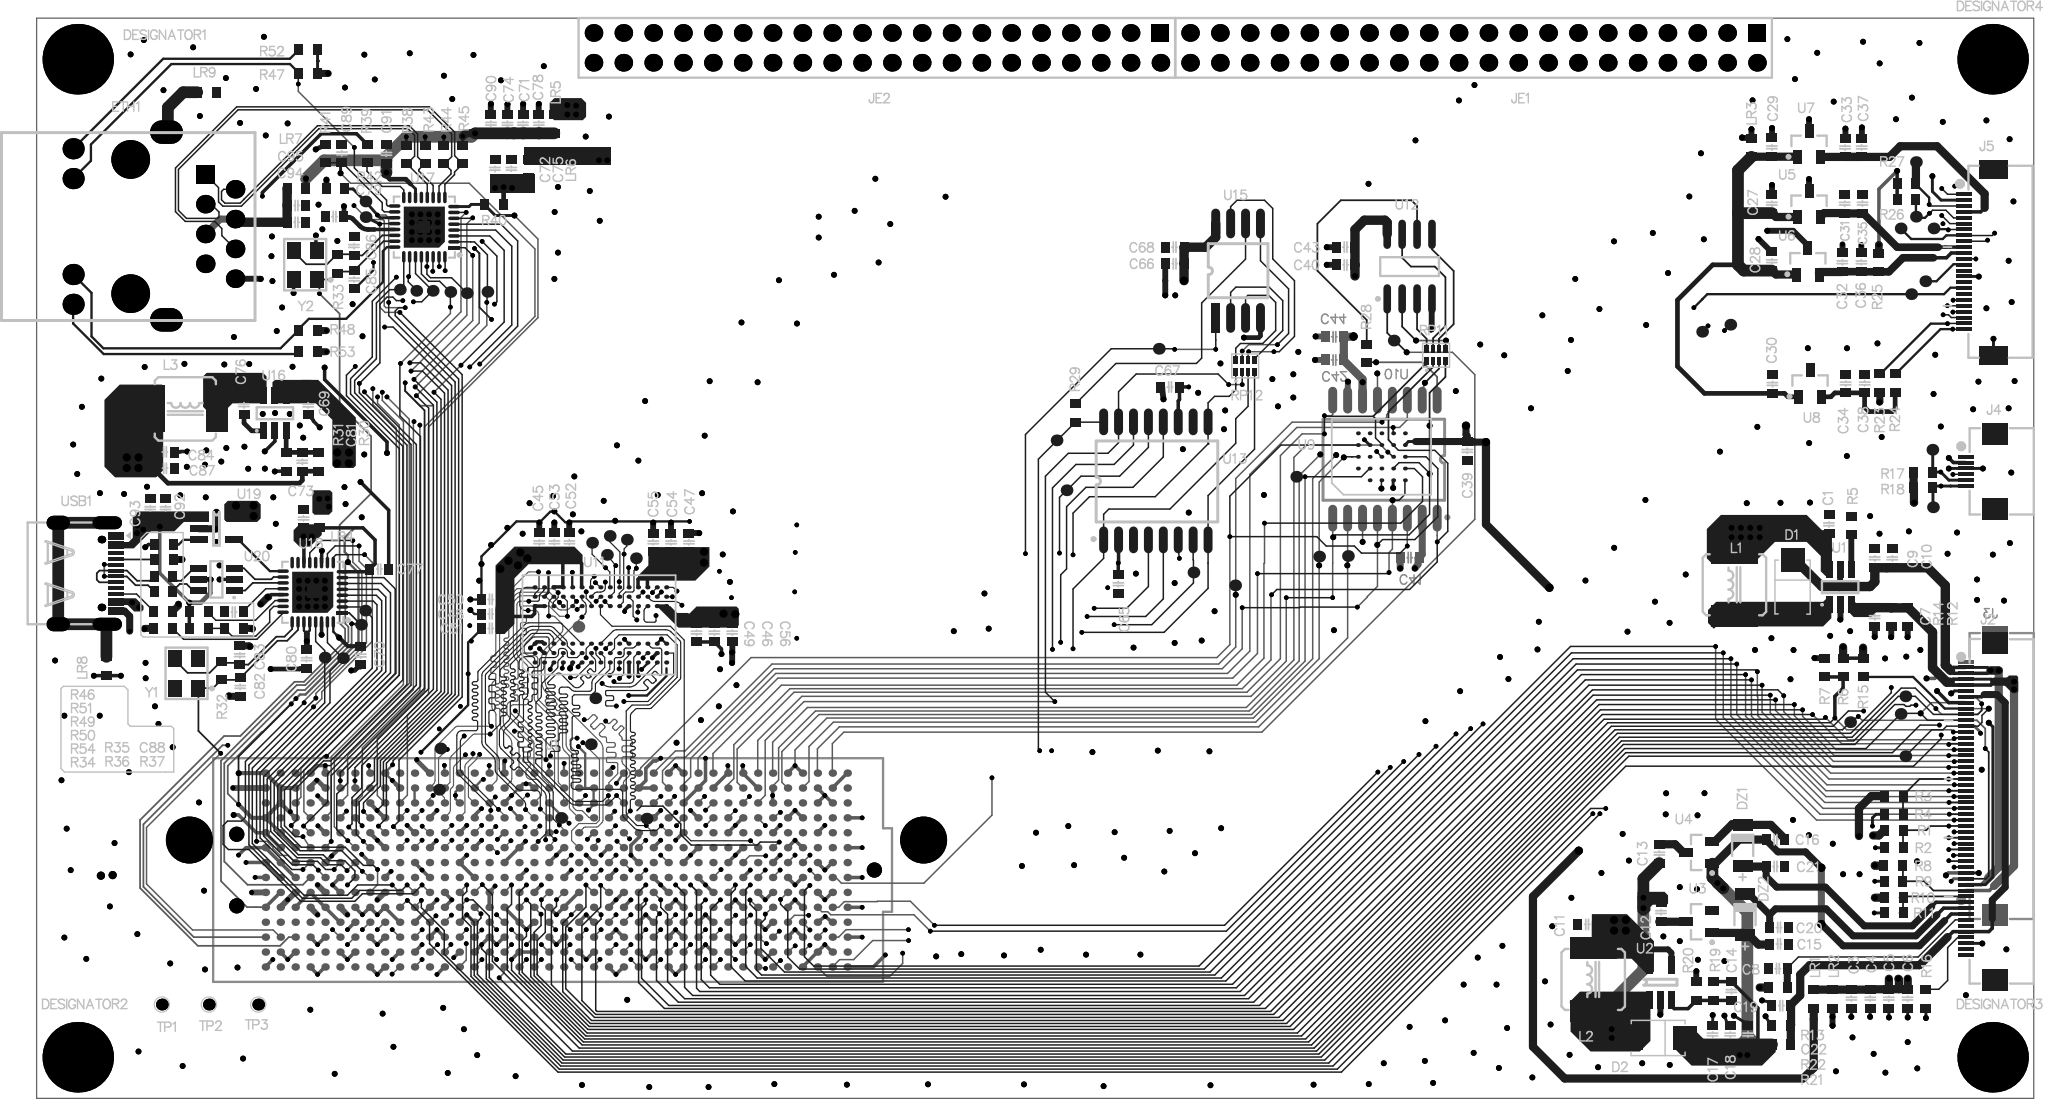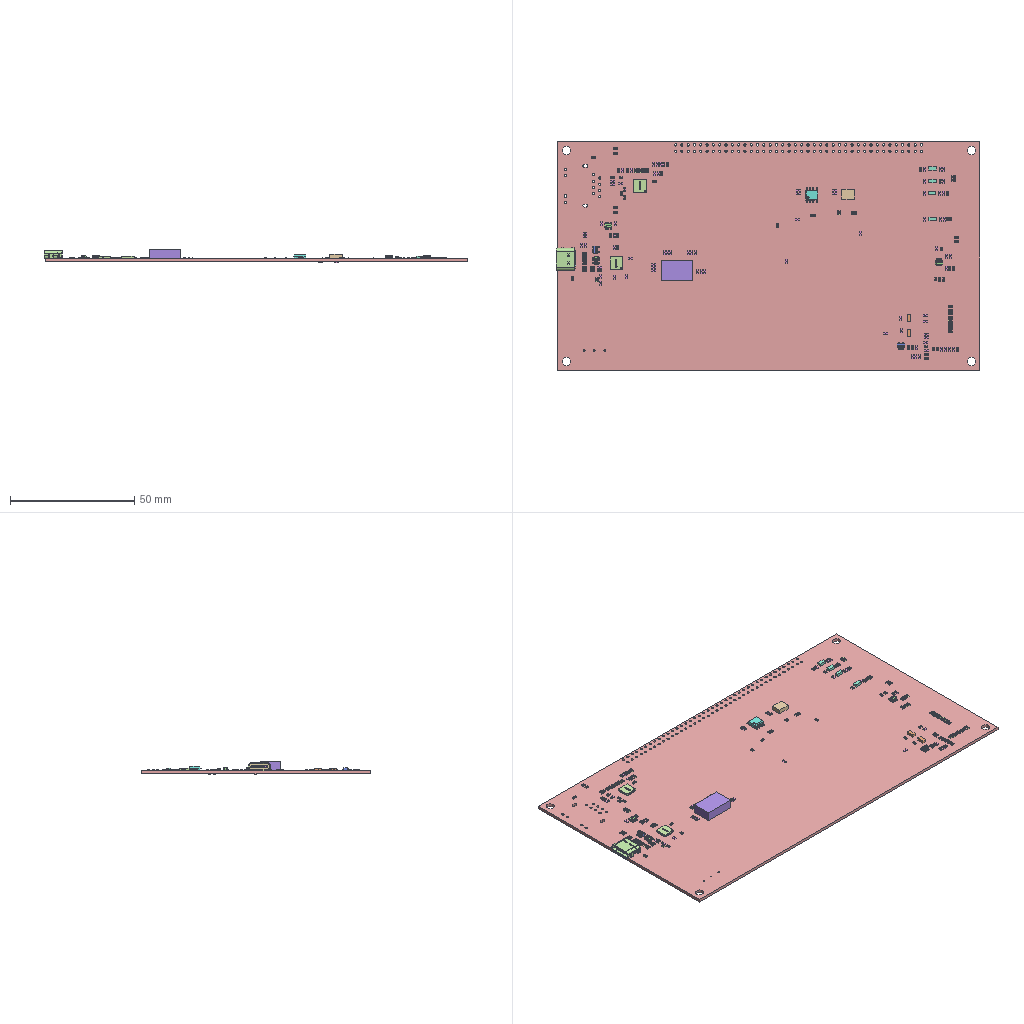Circuit board layout | Altium Designer | box 170.7 x 92 x 5.4 mm
Layer stack:
# Altium Designer layer stack of  (unit mm; dielectric type: 0 none, 1 core, 2 prepreg, 3 surface material)
index,name,kind,layer,copper_thickness_mm,dielectric_type,dielectric_thickness_mm,dielectric_material,dielectric_constant
0,Paste Mask Top,other,,,,,,
1,Silkscreen Top,other,,,,,,
2,Solder Mask Top,dielectric,,,3,0.0102,Solder Resist,3.5
3,Top,copper,Top,0.0356,,,,
4,Dielectric 1,dielectric,,,0,0.254,FR-4,4.2
5,GND,copper,GND,0.036,,,,
6,Dielectric2,dielectric,,,0,0.127,FR-4,4.2
7,mid-1,copper,mid-1,0.036,,,,
8,Dielectric3,dielectric,,,0,0.254,FR-4,4.2
9,mid-2,copper,mid-2,0.036,,,,
10,Dielectric4,dielectric,,,0,0.127,FR-4,4.2
11,mid-3,copper,mid-3,0.036,,,,
12,Dielectric5,dielectric,,,0,0.254,FR-4,4.2
13,Bottom,copper,Bottom,0.0356,,,,
14,Solder Mask Bottom,dielectric,,,3,0.0102,Solder Resist,3.5
15,Silkscreen Bottom,other,,,,,,
16,Paste Mask Bottom,other,,,,,,
# drill layer pairs: low layer,high layer
drill_pair,Top,Bottom
Part placement:
Designator,Comment,Layer,Footprint,Center-X(mm),Center-Y(mm),Rotation
Y2,XTAL_SMD3225,TopLayer,XTAL_SMD3225,3.4,59.8,90
Y1,XTAL_SMD3225$2F$2,TopLayer,XTAL_SMD3225$2F$2,-6.7,25,90
USB1,USB_TYPE-C_16PIN,TopLayer,USB_TYPE-C_16PIN,-15.17,33.51,180
U9,PBGA24_6X8,TopLayer,PBGA24_6X8,95,43.45,90
U8,SOT-23,TopLayer,SOT-23,131.484,49.686,0
U7,SOT-23,TopLayer,SOT-23,131.4,70.1,0
U6,SOT-23,TopLayer,SOT-23,131.3,60.1,0
U5,SOT-23,TopLayer,SOT-23,131.4,65,0
U4,SOT-23,TopLayer,SOT-23,122.05,9.75,90
U3,SOT-23,TopLayer,SOT-23,122.05,3.85,90
U20,SOT-23-6,TopLayer,SOT-23-6,-4.17,33.01,180
U2,SOT-23-5,TopLayer,SOT-23-5,118.75,-1.3,90
U19,SOT-23-5,TopLayer,SOT-23-5,-4.161,37.317,0
U18,QFN32_5X5,TopLayer,QFN32_5X5,4.03,31.91,90
U17,QFN32_5X5$2F$2,TopLayer,QFN32_5X5,13.53,63.01,90
U16,SOT-23-6,TopLayer,SOT-23-6,0.8117,47.161,90
U15,SOIC8,TopLayer,SOIC8,82.8,59.3,90
U13,SOIC16,TopLayer,SOIC16,75.8,41.4,90
U12,SOP8,TopLayer,SOP8,97.4,59.65,90
U11,VFBGA90_8X13,TopLayer,VFBGA90_8X13,28.52,29.133,90
U10,SOIC16,BottomLayer,SOIC16,95.3,43.25,90
U1,SOT-23-6,TopLayer,SOT-23-6,134.05,32.35,90
TP9,FZ_TP-SMD-MINI,TopLayer,FZ_TP-SMD-MINI,141.9,44.05,0
TP8,FZ_TP-SMD-MINI,TopLayer,FZ_TP-SMD-MINI,141.95,39.15,0
TP7,FZ_TP-SMD-MINI,TopLayer,FZ_TP-SMD-MINI,134.9,20.85,0
TP6,FZ_TP-SMD-MINI,TopLayer,FZ_TP-SMD-MINI,139.6,17.95,0
TP51,FZ_TP-SMD-MINI,TopLayer,FZ_TP-SMD-MINI,8.533,63.866,90
TP50,FZ_TP-SMD-MINI,TopLayer,FZ_TP-SMD-MINI,8.521,65.198,90
TP5,FZ_TP-SMD-MINI,TopLayer,FZ_TP-SMD-MINI,139.2,21.55,0
TP49,FZ_TP-SMD-MINI,TopLayer,FZ_TP-SMD-MINI,8.14,29.149,270
TP48,FZ_TP-SMD-MINI,TopLayer,FZ_TP-SMD-MINI,6.6,26.3,270
TP47,FZ_TP-SMD-MINI,TopLayer,FZ_TP-SMD-MINI,8.5,30.35,270
TP46,FZ_TP-SMD-MINI,TopLayer,FZ_TP-SMD-MINI,5.05,26.35,270
TP45,FZ_TP-SMD-MINI,TopLayer,FZ_TP-SMD-MINI,14.245,57.586,90
TP44,FZ_TP-SMD-MINI,TopLayer,FZ_TP-SMD-MINI,17.145,57.386,90
TP43,FZ_TP-SMD-MINI,TopLayer,FZ_TP-SMD-MINI,11.445,57.686,90
TP42,FZ_TP-SMD-MINI,TopLayer,FZ_TP-SMD-MINI,15.745,57.486,90
TP41,FZ_TP-SMD-MINI,TopLayer,FZ_TP-SMD-MINI,12.845,57.586,90
TP40,FZ_TP-SMD-MINI,TopLayer,FZ_TP-SMD-MINI,18.9,57.5,90
TP4,FZ_TP-SMD-MINI,TopLayer,FZ_TP-SMD-MINI,139.6,23.05,0
TP39,FZ_TP-SMD-MINI,TopLayer,FZ_TP-SMD-MINI,76.05,52.65,90
TP37,FZ_TP-SMD-MINI,TopLayer,FZ_TP-SMD-MINI,68.2,40.6,90
TP36,FZ_TP-SMD-MINI,TopLayer,FZ_TP-SMD-MINI,67.35,44.85,90
TP35,FZ_TP-SMD-MINI,TopLayer,FZ_TP-SMD-MINI,79,33.6,90
TP34,FZ_TP-SMD-MINI,TopLayer,FZ_TP-SMD-MINI,96.05,53.35,90
TP33,FZ_TP-SMD-MINI,TopLayer,FZ_TP-SMD-MINI,32.453,12.631,90
TP32,FZ_TP-SMD-MINI,TopLayer,FZ_TP-SMD-MINI,28.084,22.885,90
TP31,FZ_TP-SMD-MINI,TopLayer,FZ_TP-SMD-MINI,25.166,12.691,90
TP30,FZ_TP-SMD-MINI,BottomLayer,FZ_TP-SMD-MINI,26.646,28.973,90
TP3,FZ_TP-VIA,TopLayer,FZ_TP-VIA,-0.61,-3.2,0
TP29,FZ_TP-SMD-MINI,TopLayer,FZ_TP-SMD-MINI,27.704,18.966,90
TP28,FZ_TP-SMD-MINI,TopLayer,FZ_TP-SMD-MINI,29.312,36.708,90
TP27,FZ_TP-SMD-MINI,TopLayer,FZ_TP-SMD-MINI,29.077,35.099,90
TP26,FZ_TP-SMD-MINI,TopLayer,FZ_TP-SMD-MINI,30.77,36.392,90
TP25,FZ_TP-SMD-MINI,TopLayer,FZ_TP-SMD-MINI,31.545,34.807,90
TP24,FZ_TP-SMD-MINI,TopLayer,FZ_TP-SMD-MINI,27.81,36.126,90
TP23,FZ_TP-SMD-MINI,TopLayer,FZ_TP-SMD-MINI,14.783,15.095,90
TP22,FZ_TP-SMD-MINI,TopLayer,FZ_TP-SMD-MINI,14.902,18.61,90
TP21,FZ_TP-SMD-MINI,TopLayer,FZ_TP-SMD-MINI,92.15,35,270
TP20,FZ_TP-SMD-MINI,TopLayer,FZ_TP-SMD-MINI,82.55,32.5,90
TP2,FZ_TP-VIA,TopLayer,FZ_TP-VIA,-4.81,-3.2,0
TP19,FZ_TP-SMD-MINI,TopLayer,FZ_TP-SMD-MINI,87.75,41.75,90
TP18,FZ_TP-SMD-MINI,TopLayer,FZ_TP-SMD-MINI,89.7,34.95,90
TP17,FZ_TP-SMD-MINI,TopLayer,FZ_TP-SMD-MINI,140.1,57.3,90
TP16,FZ_TP-SMD-MINI,TopLayer,FZ_TP-SMD-MINI,141.3,58.4,90
TP15,FZ_TP-SMD-MINI,TopLayer,FZ_TP-SMD-MINI,124.7,54.7,90
TP14,FZ_TP-SMD-MINI,TopLayer,FZ_TP-SMD-MINI,140.5,63.9,90
TP13,FZ_TP-SMD-MINI,TopLayer,FZ_TP-SMD-MINI,140.5,68.55,90
TP12,FZ_TP-SMD-MINI,TopLayer,FZ_TP-SMD-MINI,122.3,54.1,90
TP11,FZ_TP-SMD-MINI,TopLayer,FZ_TP-SMD-MINI,139.2,62.9,90
TP10,FZ_TP-SMD-MINI,TopLayer,FZ_TP-SMD-MINI,142,62.9,90
TP1,FZ_TP-VIA,TopLayer,FZ_TP-VIA,-8.81,-3.2,0
RP12,0402RP-4P,TopLayer,0402RP-4P,83.4,51.2,0
RP11,0402RP-4P,TopLayer,0402RP-4P,99.65,52.1,0
R9,0603R_N,TopLayer,0603R_N,138.593,7.3,0
R8,0603R_N,TopLayer,0603R_N,138.568,8.625,180
R7,0603R_N,TopLayer,0603R_N,132.75,25.5,270
R6,0603R_N,TopLayer,0603R_N,134.3,25.5,90
R54,0603R_N,TopLayer,0603R_N,-8.691,30.236,180
R53,0603R_N,TopLayer,0603R_N,3.6,52.4,180
R52,0603R_N,TopLayer,0603R_N,3.643,78.103,180
R51,0603R_N,TopLayer,0603R_N,-8.655,34.705,180
R50,0603R_N,TopLayer,0603R_N,-8.67,31.985,180
R5,0603R_N,TopLayer,0603R_N,135.05,37.6,270
R49,0603R_N,TopLayer,0603R_N,-8.67,33.26,180
R48,0603R_N,TopLayer,0603R_N,3.6,54.2,180
R47,0603R_N,TopLayer,0603R_N,3.643,76.103,180
R46,0603R_N,TopLayer,0603R_N,-8.655,35.98,0
R45,0603R_N,TopLayer,0603R_N,16.8,69.2,90
R44,0603R_N,TopLayer,0603R_N,15.2,69.2,90
R43,0603R_N,TopLayer,0603R_N,13.6,69.2,90
R42,0603R_N,TopLayer,0603R_N,5.977,66.262,0
R41,0603R_N,TopLayer,0603R_N,5.103,69.289,270
R40,0603R_N,TopLayer,0603R_N,19.479,64.943,180
R4,0603R_N,TopLayer,0603R_N,138.6,13,0
R39,0603R_N,TopLayer,0603R_N,8.652,69.272,270
R38,0603R_N,TopLayer,0603R_N,12,69.2,90
R37,0603R_N,TopLayer,0603R_N,-2.692,28.836,0
R36,0603R_N,TopLayer,0603R_N,-5.674,28.836,180
R35,0603R_N,TopLayer,0603R_N,-5.674,30.236,180
R34,0603R_N,TopLayer,0603R_N,-8.691,28.836,180
R33,0603R_N,TopLayer,0603R_N,6.15,59.9,270
R32,0603R_N,TopLayer,0603R_N,-3.7,25.25,270
R31,0603R_N,TopLayer,0603R_N,1.771,43.025,270
R30,0603R_N,TopLayer,0603R_N,4.521,43.025,90
R3,0603R_N,TopLayer,0603R_N,138.6,14.55,180
R29,0603R_N,TopLayer,0603R_N,69,47.2,270
R28,0603R_N,TopLayer,0603R_N,93.75,52.25,270
R27,0603R_N,TopLayer,0603R_N,139.7,66.7,180
R26,0603R_N,TopLayer,0603R_N,139.7,65.4,180
R25,0603R_N,TopLayer,0603R_N,137.343,60.003,90
R24,0603R_N,TopLayer,0603R_N,138.73,49.71,90
R23,0603R_N,TopLayer,0603R_N,137.43,49.71,90
R22,0603R_N,TopLayer,0603R_N,129.038,-4.988,0
R21,0603R_N,TopLayer,0603R_N,129.05,-6.6,180
R20,0603R_N,TopLayer,0603R_N,121.8,-2.05,270
R2,0603R_N,TopLayer,0603R_N,138.6,10.15,0
R19,0603R_N,TopLayer,0603R_N,123.25,-2.05,90
R18,0603R_N,TopLayer,0603R_N,141.13,40.81,180
R17,0603R_N,TopLayer,0603R_N,141.13,42.11,180
R16,0603R_N,TopLayer,0603R_N,141.35,-2.7,90
R15,0603R_N,TopLayer,0603R_N,136,25.5,90
R14,0603R_N,TopLayer,0603R_N,138.4,29.782,90
R13,0603R_N,TopLayer,0603R_N,128.75,-1.75,180
R12,0603R_N,TopLayer,0603R_N,139.8,29.782,90
R11,0603R_N,TopLayer,0603R_N,138.6,4.6,0
R10,0603R_N,TopLayer,0603R_N,138.6,5.9,180
R1,0603R_N,TopLayer,0603R_N,138.6,11.65,180
LR9,0603R_N,TopLayer,0603R_N,-5,74.5,180
LR8,0603R_N,TopLayer,0603R_N,-13.53,25.612,90
LR7,0603R_N,TopLayer,0603R_N,2.652,66.34,180
LR6,0603R_N,TopLayer,0603R_N,22.4,68,90
LR5,0603R_N,TopLayer,0603R_N,24.6,71.8,90
LR4,0603R_N,TopLayer,0603R_N,4.566,38.197,90
LR3,0603R_N,TopLayer,0603R_N,126.5,69.8,90
LR2,0603R_N,TopLayer,0603R_N,133.4,-2.7,270
LR1,0603R_N,TopLayer,0603R_N,131.8,-2.7,270
L3,LD-5.5MM,TopLayer,LD-5.5MM,-6.814,47.528,180
L2,LD-5.5MM$2F$2,TopLayer,LD-5.5mm,113.029,-1.065,270
L1,LD-5.5MM$2F$3,TopLayer,LD-5.5mm,125.05,32.55,270
JE2,HDR2X20,TopLayer,HDR2X20,52.06,78.28,180
JE1,HDR2X20,TopLayer,HDR2X20,102.84,78.28,180
J5,FPC0.5-24P,TopLayer,,145.879,60.033,90
J4,FPC0.5-6P,TopLayer,,145.982,42.21,90
J3,FPC0.5-40P,BottomLayer,,145.978,16.26,270
J2,FPC0.5-50P,TopLayer,,145.978,13.21,90
J1,ASP-184330-01_BOTTOM,TopLayer,ASP-184330-01_BOTTOM,24.765,8.255,180
ETH1,RJ45_HR911003A,TopLayer,RJ45_HR911003A,-9.47,63.11,270
DZ2,LL-34,TopLayer,LL-34,125.95,4.45,90
DZ1,LL-34,TopLayer,LL-34,125.75,10.35,90
DESIGNATOR4,FZ_HOLE_M3.4,TopLayer,FZ_HOLE_M3.4,147.03,77.31,0
DESIGNATOR3,FZ_HOLE_M3.4,TopLayer,FZ_HOLE_M3.4,147.03,-7.69,0
DESIGNATOR2,FZ_HOLE_M3.4,TopLayer,FZ_HOLE_M3.4,-15.97,-7.69,0
DESIGNATOR1,FZ_HOLE_M3.4,TopLayer,FZ_HOLE_M3.4,-15.97,77.31,0
D2,DO-214AC,TopLayer,DO-214AC,118.55,-6.05,0
D1,DO-214AC,TopLayer,DO-214AC,130,32.35,90
C95,0603C_N,TopLayer,0603C_N,2.652,64.862,180
C94,0603C_N,TopLayer,0603C_N,2.652,63.427,180
C93,0603C_N,TopLayer,0603C_N,-9.792,39.075,90
C92,0603C_N,TopLayer,0603C_N,-8.492,39.075,90
C91,0603C_N,TopLayer,0603C_N,10.286,69.252,270
C90,0603C_N,TopLayer,0603C_N,19.187,71.813,270
C9,0603C_N,TopLayer,0603C_N,137,34.8,90
C89,0603C_N,TopLayer,0603C_N,6.503,69.289,270
C88,0603C_N,TopLayer,0603C_N,-2.692,30.236,180
C87,0603C_N,TopLayer,0603C_N,-8.545,42.483,180
C86,0603C_N,TopLayer,0603C_N,7.55,61.4,90
C85,0603C_N,TopLayer,0603C_N,7.55,58.55,270
C84,0603C_N,TopLayer,0603C_N,-8.545,43.857,0
C83,0603C_N,TopLayer,0603C_N,-2.174,26.55,90
C82,0603C_N,TopLayer,0603C_N,-2.15,23.85,270
C81,0603C_N,TopLayer,0603C_N,3.146,43.025,90
C80,0603C_N,TopLayer,0603C_N,3.492,26.219,270
C8,0603C_N,TopLayer,0603C_N,128.75,-0.1501,0
C79,0603C_N,TopLayer,0603C_N,5.892,63.899,0
C78,0603C_N,TopLayer,0603C_N,23.267,71.814,270
C77,0603C_N,TopLayer,0603C_N,9.698,33.893,180
C76,0603C_N,TopLayer,0603C_N,-1.819,47.847,90
C75,0603C_N,TopLayer,0603C_N,20.924,67.974,270
C74,0603C_N,TopLayer,0603C_N,20.6,71.8,270
C73,0603C_N,TopLayer,0603C_N,3.24,38.194,270
C72,0603C_N,TopLayer,0603C_N,19.549,67.974,90
C71,0603C_N,TopLayer,0603C_N,21.934,71.814,90
C70,0603C_N,TopLayer,0603C_N,8.117,26.52,270
C7,0603C_N,TopLayer,0603C_N,137,29.8,90
C69,0603C_N,TopLayer,0603C_N,3.637,47.816,270
C68,0603C_N,TopLayer,0603C_N,77.4,61.3,0
C67,0603C_N,TopLayer,0603C_N,77.013,49.387,0
C66,0603C_N,TopLayer,0603C_N,77.4,59.9,180
C65,0603C_N,TopLayer,0603C_N,72.6,32.6,270
C6,0603C_N,TopLayer,0603C_N,139.8,-2.7,90
C56,0603C_N,TopLayer,0603C_N,39.748,28.479,90
C55,0603C_N,TopLayer,0603C_N,33.006,36.159,270
C54,0603C_N,TopLayer,0603C_N,34.526,36.159,270
C53,0603C_N,TopLayer,0603C_N,24.59,36.165,270
C52,0603C_N,TopLayer,0603C_N,25.863,36.165,270
C51,0603C_N,TopLayer,0603C_N,19.193,28.825,0
C50,0603C_N,TopLayer,0603C_N,19.193,31.295,0
C5,0603C_N,TopLayer,0603C_N,138.2,-2.7,90
C49,0603C_N,TopLayer,0603C_N,36.708,28.479,90
C48,0603C_N,TopLayer,0603C_N,19.193,30.06,0
C47,0603C_N,TopLayer,0603C_N,36.046,36.159,270
C46,0603C_N,TopLayer,0603C_N,38.228,28.479,90
C45,0603C_N,TopLayer,0603C_N,23.317,36.165,90
C44,0603C_N,BottomLayer,0603C_N,91,53.675,0
C43,0603C_N,TopLayer,0603C_N,91.95,61.3,0
C42,0603C_N,BottomLayer,0603C_N,91,51.7,0
C41,0603C_N,BottomLayer,0603C_N,97.4,34.85,180
C40,0603C_N,TopLayer,0603C_N,91.95,59.8,180
C4,0603C_N,TopLayer,0603C_N,136.6,-2.7,270
C39,0603C_N,TopLayer,0603C_N,102.3,43.95,270
C38,0603C_N,TopLayer,0603C_N,136.13,49.694,270
C37,0603C_N,TopLayer,0603C_N,135.87,69.79,270
C36,0603C_N,TopLayer,0603C_N,135.846,60.008,270
C35,0603C_N,TopLayer,0603C_N,135.946,65.008,270
C34,0603C_N,TopLayer,0603C_N,134.53,49.694,90
C33,0603C_N,TopLayer,0603C_N,134.47,69.79,90
C32,0603C_N,TopLayer,0603C_N,134.243,60.017,90
C31,0603C_N,TopLayer,0603C_N,134.446,65.008,90
C30,0603C_N,TopLayer,0603C_N,128.3,49.65,90
C3,0603C_N,TopLayer,0603C_N,135,-2.7,270
C29,0603C_N,TopLayer,0603C_N,128.246,69.808,90
C28,0603C_N,TopLayer,0603C_N,128.246,60.108,90
C27,0603C_N,TopLayer,0603C_N,128.246,65.008,90
C22,0603C_N,TopLayer,0603C_N,129.038,-3.288,180
C21,0603C_N,TopLayer,0603C_N,128.55,8.55,0
C20,0603C_N,TopLayer,0603C_N,128.85,3.35,0
C19,0603C_N,TopLayer,0603C_N,126.2,-5.75,270
C18,0603C_N,TopLayer,0603C_N,124.7,-5.75,90
C17,0603C_N,TopLayer,0603C_N,123.2,-5.75,90
C16,0603C_N,TopLayer,0603C_N,128.55,10.85,180
C15,0603C_N,TopLayer,0603C_N,128.85,1.95,0
C14,0603C_N,TopLayer,0603C_N,124.8,-2.05,90
C13,0603C_N,TopLayer,0603C_N,118.65,9.65,270
C12,0603C_N,TopLayer,0603C_N,118.806,4.674,90
C11,0603C_N,TopLayer,0603C_N,112.512,3.633,180
C10,0603C_N,TopLayer,0603C_N,138.5,34.8,90
C1,0603C_N,TopLayer,0603C_N,133.1,37.7,90
Pad and via stacks:
# Altium Designer via and pad stacks of  (unit mm). Each distinct definition once, with the count of objects using it.
# via: kind,start_layer,end_layer,hole_mm,diameter_mm,mode(0 simple;1 top-mid-bottom;2 full stack),diameter_per_layer,count,example_net
# pad: kind,layer,hole_mm,hole_type(0 round;1 square;2 slot),plating,top_size,top_shape(1 round;2 rect;3 octagon;9 rounded rect),mid_size,bottom_size,mode,footprint,size_per_layer,count,example
pad,Top,0,0,plated,1.8x4,2,1.8x4,1.8x4,0,LD-5.5mm,,6,L2.2
pad,Top,0,0,plated,0.3556x0.3556,1,0.3556x0.3556,0.3556x0.3556,0,VFBGA90_8X13,,90,U11.K7
pad,Top,0,0,plated,0.762x0.8636,2,0.762x0.8636,0.762x0.8636,0,0603C_N,,158,C1.2
pad,Top,0,0,plated,2x2,2,2x2,2x2,0,DO-214AC,,4,D1.1
pad,Top,0,0,unplated,1.65x0.95,2,1.65x0.95,1.65x0.95,0,LL-34,,4,DZ1.1
pad,Top,0,0,plated,0.762x0.8636,2,0.762x0.8636,0.762x0.8636,0,0603R_N,,126,LR1.1
pad,Top,0,0,plated,0.3x0.6,2,0.3x0.6,0.3x0.6,0,0402RP-4P,,8,RP11.2
pad,Top,0,0,plated,0.4x0.6,2,0.4x0.6,0.4x0.6,0,0402RP-4P,,8,RP11.1
pad,Top,0,0,plated,1x1,1,1x1,1x1,0,FZ_TP-SMD-MINI,,46,TP10.1
pad,Top,0,0,plated,0.7x1.15,2,0.7x1.15,0.7x1.15,0,SOT-23,,18,U3.3
pad,Top,0,0,plated,0.65x2.5,1,0.65x2.5,0.65x2.5,0,SOP8,,8,U12.5
pad,Top,0,0,plated,2.286x0.762,1,2.286x0.762,2.286x0.762,0,SOIC16,,16,U13.16
pad,Top,0,0,plated,2.54x0.762,1,2.54x0.762,2.54x0.762,0,SOIC8,,7,U15.5
pad,Top,0,0,plated,2.54x0.762,2,2.54x0.762,2.54x0.762,0,SOIC8,,1,U15.1
pad,Top,0,0,unplated,1x1,2,1x1,1x1,0,QFN32 5X5,,2,U17.0
pad,Top,0,0,plated,1x0.3,1,1x0.3,1x0.3,0,QFN32 5X5,,62,U17.32
pad,Top,0,0,plated,1x0.3,2,1x0.3,1x0.3,0,QFN32 5X5,,2,U17.1
pad,Top,0,0,plated,1.5x0.52,2,1.5x0.52,1.5x0.52,0,SOT-23-5,,10,U19.4
pad,Top,0,0,plated,0.55x1.4,2,0.55x1.4,0.55x1.4,0,SOT-23-6,,18,U1.6
pad,Top,0,0,plated,0.6x1.3,2,0.6x1.3,0.6x1.3,0,USB_TYPE-C_16PIN,,4,USB1.12
pad,Top,0,0,plated,0.3x1.3,2,0.3x1.3,0.3x1.3,0,USB_TYPE-C_16PIN,,8,USB1.3
pad,Top,0,0,unplated,1.4x1.15,2,1.4x1.15,1.4x1.15,0,XTAL_SMD3225,,4,Y2.4
pad,Top,0,0,unplated,1.4x1.15,2,1.4x1.15,1.4x1.15,0,XTAL_SMD3225$2F$2,,4,Y1.4
pad,Top,0,0,plated,0.3302x0.3302,1,0.3302x0.3302,0.3302x0.3302,0,PBGA24_6X8,,24,U9.E5
pad,Top,0,0,plated,1.3x0.3,2,1.3x0.3,1.3x0.3,0,,,80,J5.24
pad,Top,0,0,plated,2.4x1.6,2,2.4x1.6,2.4x1.6,0,,,2,J5.0/2
pad,Top,0,0,plated,2.2x1.8,2,2.2x1.8,2.2x1.8,0,,,4,J4.0/2
pad,Bottom,0,0,plated,0.64x0.64,1,0.64x0.64,0.64x0.64,0,ASP-184330-01_BOTTOM,,560,J1.L1
pad,Bottom,0,0,plated,0.762x0.8636,2,0.762x0.8636,0.762x0.8636,0,0603C_N,,6,C41.2
pad,Bottom,0,0,plated,1x1,1,1x1,1x1,0,FZ_TP-SMD-MINI,,1,TP30.1
pad,Bottom,0,0,plated,2.286x0.762,1,2.286x0.762,2.286x0.762,0,SOIC16,,16,U10.16
pad,Bottom,0,0,plated,1.3x0.3,2,1.3x0.3,1.3x0.3,0,,,40,J3.40
pad,Bottom,0,0,plated,2.2x1.8,2,2.2x1.8,2.2x1.8,0,,,2,J3.0/2
pad,Multi-Layer,3.4,0,plated,6x6,1,6x6,6x6,0,FZ_HOLE_M3.4,,4,DESIGNATOR1.1
pad,Multi-Layer,0.889,0,plated,1.575x1.575,1,1.575x1.575,1.575x1.575,0,RJ45_HR911003A,,7,ETH1.5
pad,Multi-Layer,0.889,0,plated,1.575x1.575,2,1.575x1.575,1.575x1.575,0,RJ45_HR911003A,,1,ETH1.1
pad,Multi-Layer,1.2,2,plated,2x2.8,1,2x2.8,2x2.8,0,RJ45_HR911003A,,2,ETH1.SH1
pad,Multi-Layer,1.02,0,plated,1.8x1.8,1,1.8x1.8,1.8x1.8,0,RJ45_HR911003A,,4,ETH1.9
pad,Multi-Layer,0.9,0,plated,1.5x1.5,2,1.5x1.5,1.5x1.5,0,HDR2X20,,2,JE1.1
pad,Multi-Layer,0.9,0,plated,1.5x1.5,1,1.5x1.5,1.5x1.5,0,HDR2X20,,78,JE1.2
pad,Multi-Layer,0.6,0,plated,1x1,1,1x1,1x1,0,FZ_TP-VIA,,3,TP1.1
pad,Multi-Layer,0.6,2,plated,1.2x2,1,1.2x2,1.2x2,0,USB_TYPE-C_16PIN,,2,USB1.S4
pad,Multi-Layer,0.6,2,plated,1.1x2.5,1,1.1x2.5,1.1x2.5,0,USB_TYPE-C_16PIN,,2,USB1.S3
pad,Multi-Layer,0.65,0,unplated,0.65x0.65,1,0.65x0.65,0.65x0.65,0,USB_TYPE-C_16PIN,,2,USB1.
via,Top,Bottom,0.2,0.4,0,,618,GND
via,Top,Bottom,1.3,1.3,0,,3,
via,Top,Bottom,0.3,0.5,0,,563,GND
via,Top,Bottom,0.4,0.7,0,,34,+3_3V
via,Top,Bottom,4,4,0,,2,
via,Top,Bottom,3.3,3.3,0,,2,
via,Top,Bottom,0.5,1,0,,36,
Copper pours:
name,layer,net,type(0 solid;1 hatched;2 none)
NONET_L03_P010,mid-1,,0
NONET_L03_P000,mid-1,,0
NONET_L05_P005,mid-3,,0
NONET_L05_P006,mid-3,,0
NONET_L05_P011,mid-3,,0
NONET_L05_P007,mid-3,,0
NONET_L05_P003,mid-3,,0
NONET_L05_P004,mid-3,,0
NONET_L05_P002,mid-3,,0
NONET_L05_P001,mid-3,,0
NONET_L01_P008,Top,,0
NONET_L02_P009,GND,,0
NONET_L06_P012,Bottom,,0
NONET_L04_P013,mid-2,,0
Design rules, without the lines most boards share:
# Altium Designer design rules of  (exported by Altium Designer, unit mm)
# columns: name | kind | enabled | priority | scope1 | scope2 | descriptor | typed fields (field=value)
Clearance | 0 | enabled | 1 | InNet('NETETH1_SH1') | All | Clearance Constraint (Gap=0.5mm) (InNet('NETETH1_SH1')),(All) | gap=0.5
DiffPairsRouting | 51 | enabled | 1 | All | All | Differential Pairs Uncoupled Length using the Gap Constraints (Min=0.254mm) (Max=0.254mm) (Prefered=0.254mm)  and Width Constraints (Min=0.381mm) (Max=0.381mm) (Prefered=0.381mm) (All) |
PlaneClearance | 12 | enabled | 1 | All | All | Power Plane Clearance (Clearance =0.508mm) (All) | clearance=0.508
Fanout_SOIC | 49 | enabled | 1 | IsSOIC | All | Fanout Control Rule ( (IsSOIC) ) |
Fanout_Small | 49 | enabled | 2 | (CompPinCount < 5) | All | Fanout Control Rule ( ((CompPinCount < 5)) ) |
SilkToSolderMaskClearance | 54 | enabled | 1 | IsPad | All | Silk To Solder Mask (Clearance=0.254mm) (IsPad),(All) |
Fanout_BGA | 49 | enabled | 3 | IsBGA | All | Fanout Control Rule ( (IsBGA) ) |
PolygonConnect - Default SMT | 20 | enabled | 1 | IsSMTPin | All | Polygon Connect Rule(Relief Connect )(Conductor Width=0.254mm) (Relief Angle=45 Angle) (Entries=4) (Air Gap Width=0.254mm) (IsSMTPin),(All) | connect_style(0=relief,1=direct,2=none)=0 relief_conductor_width=0.254 relief_entries=4
Fanout_LCC | 49 | enabled | 4 | IsLCC | All | Fanout Control Rule ( (IsLCC) ) |
Width - Net - +3_3V | 2 | enabled | 1 | InNet('+3_3V') | All | Width Constraint (Min=0.1mm) (Max=2mm) (Preferred=0.8mm) (InNet('+3_3V')) |
Width - Net - +12V | 2 | enabled | 2 | InNet('+12V') | All | Width Constraint (Min=0.1mm) (Max=2mm) (Preferred=0.5mm) (InNet('+12V')) |
Width - Net - +3_3V_ETH | 2 | enabled | 3 | InNet('+3_3V_ETH') | All | Width Constraint (Min=0.1mm) (Max=2mm) (Preferred=1mm) (InNet('+3_3V_ETH')) |
Default Length | 3 | enabled | 1 | All | All | Length Constraint (Min=0mm) (Max=1270mm) (All) |
RoutingVias - Default - DEFAULT | 11 | enabled | 1 | All | All | Routing Via (MinHoleWidth=0.2mm) (MaxHoleWidth=0.4mm) (PreferredHoleWidth=0.3mm) (MinWidth=0.4mm) (MaxWidth=0.7mm) (PreferedWidth=0.5mm) (All) | via_min_hole=0.2 via_max_hole=0.4 via_preferred_diameter=0.5 via_preferred_hole=0.3
RoutingLayers - Default - DEFAULT | 9 | enabled | 1 | All | All | Routing Layers(All) |
Default Parallel Segment Same Layer | 1 | enabled | 1 | All | All | Parallel Segment Constraint (Gap=5.08mm ) (Limit=25.4mm) (All),(All) |
Default Impedance | 33 | enabled | 1 | All | All | Impedance (Minimum=50.00Ohms Maximum=150.0Ohms) |
Default Parallel Segment Adjasent | 1 | enabled | 2 | All | All | Parallel Segment Constraint (Gap=5.08mm ) (Limit=25.4mm) (All),(All) |
HoleToHoleClearance - Default - DEFAULT | 52 | enabled | 1 | All | All | Hole To Hole Clearance (Gap=0.203mm) (All),(All) | gap=0.2032
PolygonConnect - Default Pad | 20 | enabled | 2 | All | All | Polygon Connect Rule(Relief Connect )(Conductor Width=0.254mm) (Relief Angle=45 Angle) (Entries=4) (Air Gap Width=0.254mm) (All),(All) | connect_style(0=relief,1=direct,2=none)=0 relief_conductor_width=0.254 relief_entries=4
Default PlaneConnect | 6 | enabled | 1 | All | All | Power Plane Connect Rule(Relief Connect )(Expansion=0.508mm) (Conductor Width=0.254mm) (Air Gap=0.254mm) (Entries=4) (All) | relief_conductor_width=0.254 relief_entries=4 relief_expansion=0.508
Clearance - Default - DEFAULT - Net | 0 | enabled | 2 | All | All | Clearance Constraint (Gap=0.2mm) (All),(All) | gap=0.2
ComponentClearance - Default - DEFAULT | 24 | enabled | 1 | All | All | Component Clearance Constraint ( Horizontal Gap = 0.254mm, Vertical Gap = 0.254mm ) (All),(All)  | gap=0.254
Default Width | 2 | enabled | 4 | All | All | Width Constraint (Min=0.1mm) (Max=2mm) (Preferred=0.127mm) (All) |
SMDToCorner - Default - DEFAULT | 23 | enabled | 1 | All | All | SMD To Corner (Distance=0.1mm) (All) |
RoutingPriority - Default - DEFAULT | 8 | enabled | 1 | All | All | TRoutingPriorityRule(Priority=2) (All) |
SolderMaskExpansion | 13 | enabled | 1 | All | All | Solder Mask Expansion (Expansion =0.102mm) (All) | expansion=0.1016
PasteMaskExpansion | 14 | enabled | 1 | All | All | Paste Mask Expansion (Expansion =0mm) (All) | expansion=0
RoutingCorners | 10 | enabled | 1 | All | All | Routing Corners (Style=45-Degree) (Min Setback=2.54mm) (Max Setback=2.54mm) (All) |
Height | 50 | enabled | 1 | All | All | Height Constraint (Min=0mm) (Max=25.4mm) (Prefered=12.7mm) (All) | min_height=0 max_height=25.4
NetAntennae | 56 | enabled | 1 | All | All | Net Antennae (Tolerance=0mm) (All) |
Default Routing Topology | 7 | enabled | 1 | All | All | Routing Topology Rule(Topology=Daisy_Balanced) (All) |
SilkToSilkClearance | 55 | enabled | 1 | All | All | Silk to Silk (Clearance=0.254mm) (All),(All) |
HoleSize | 42 | enabled | 1 | All | All | Hole Size Constraint (Min=0.025mm) (Max=2.54mm) (All) |
MinimumSolderMaskSliver | 53 | enabled | 1 | All | All | Minimum Solder Mask Sliver (Gap=0.254mm) (All),(All) |
Classes set for this board:
# Altium Designer classes of  (member kind: 0 net, 1 component, 2 from-to, 3 pad, 4 layer, 5 differential pair, 6 design channel, 7 polygon, 8 structure, 9 xSignal)
# columns: class name | member kind | superclass | members
RoutingClass_7(RuleSet) | 0 | no | +12V; +3_3V;